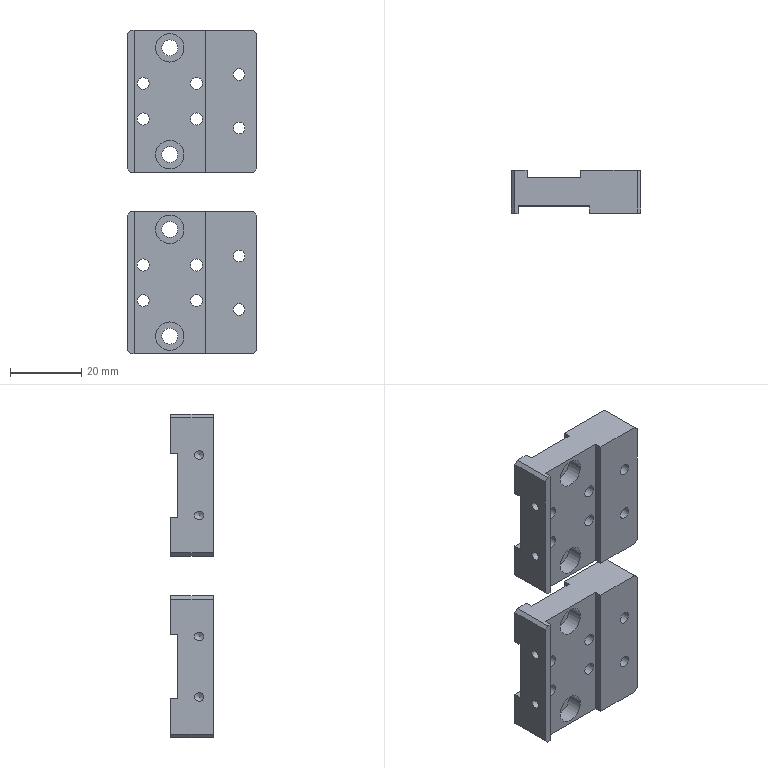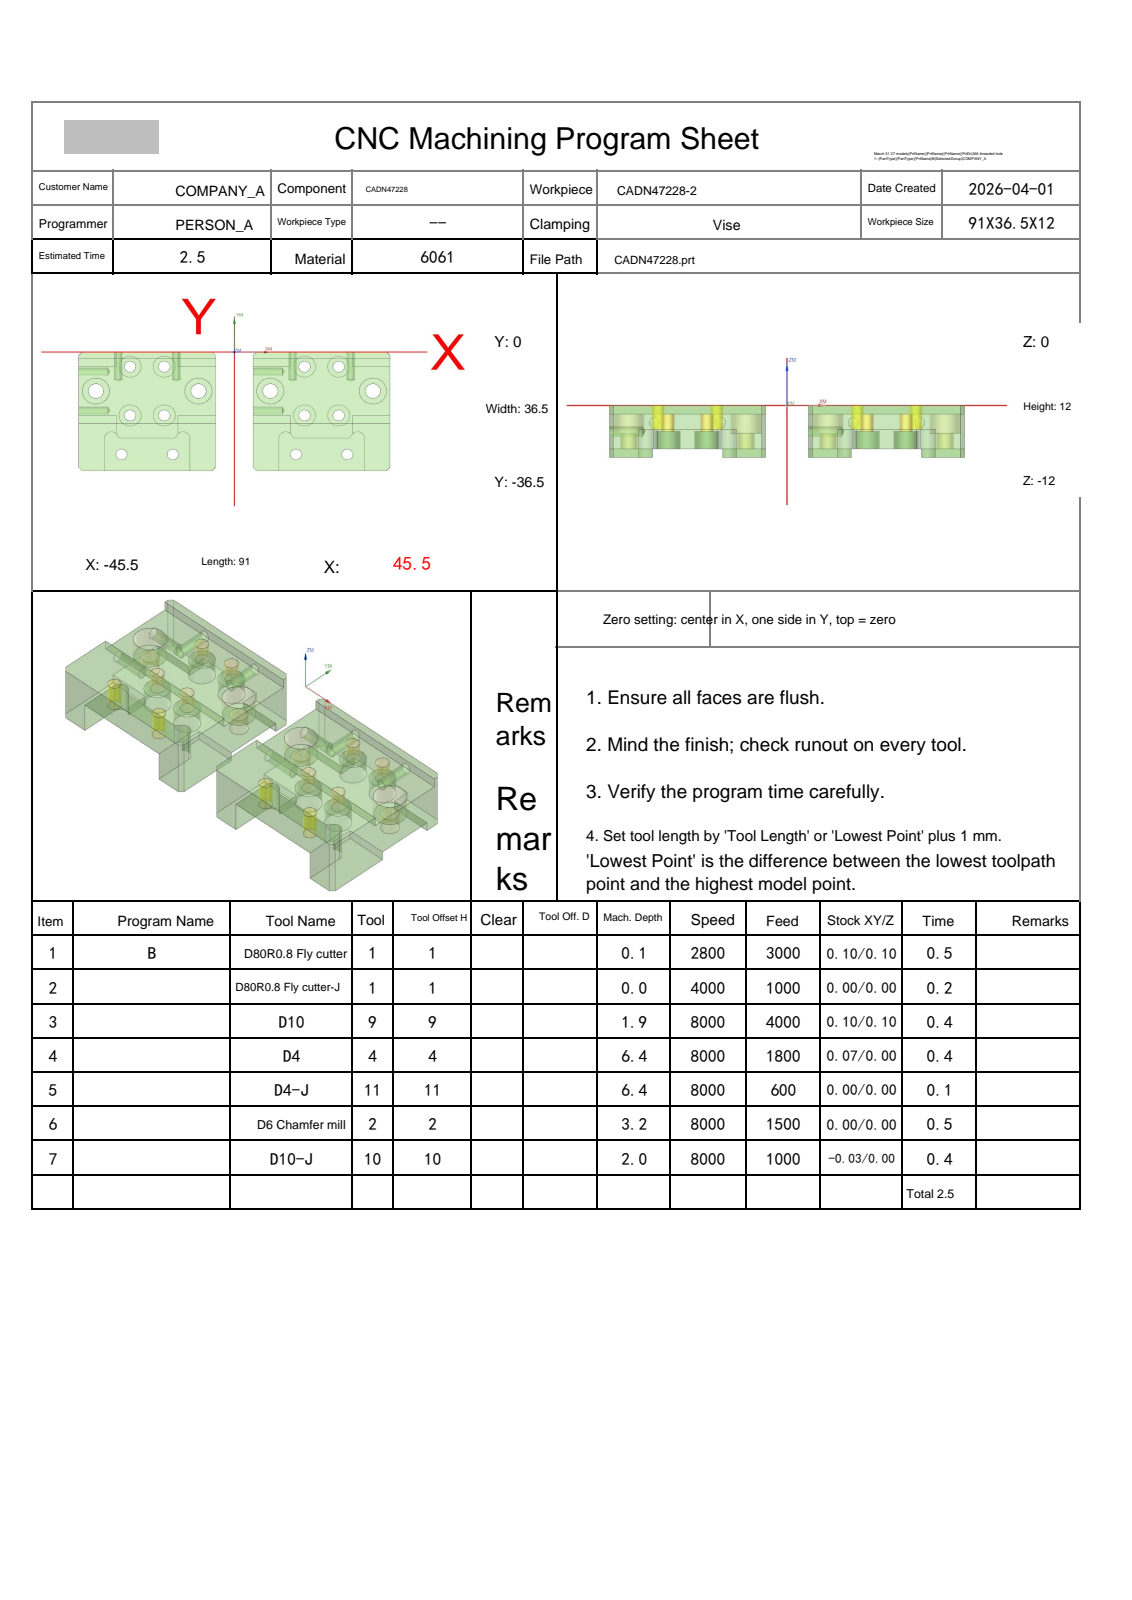NC program | NX | posted by the shop | part box 36.5 x 12 x 91 mm
Whole program:
%
O0001
(Machine time: 4.05 MIN)
(===Total Tool:6===)
(T1=D80R0.8 Fly cutter D=80.  R=0.8  D-  H01 Z=-0.   )
(T9=D10     D=10.  R=0.   D-  H09 Z=-1.9  )
(T4=D4      D=4.   R=0.   D-  H04 Z=-6.4  )
(T11=D4-J   D=4.   R=0.   D-  H11 Z=-6.4  )
(T2=D6 Chamfer mill   D=6.   R=0.   D-  H02 Z=-3.2  )
(T10=D10-J  D=10.  R=0.   D10 H10 Z=-2.   )
G80 G90 G17 G49 G40
G91 G28 Z0
M01
N1 T01 M06
(D80R0.8 Fly cutter  D=80. R=0.8 H=01 ce=0.10 di=0.10)
G00 G90 G54 X-97.597 Y-18.25 M03 S2800
G43 H01 Z20.
M08
Z4.517
G01 Z2.517 F3000.
X-85.597
X85.597
X97.597
Z4.517
G00 X-97.597
Z4.033
G01 Z2.033
X-85.597
X85.597
X97.597
Z4.033
G00 X-97.597
Z3.55
G01 Z1.55
X-85.597
X85.597
X97.597
Z3.55
G00 X-97.597
Z3.067
G01 Z1.067
X-85.597
X85.597
X97.597
Z3.067
G00 Z20.
X-97.597
Z2.583
G01 Z.583
X-85.597
X85.597
X97.597
Z2.583
G00 Z20.
X-97.597
Z2.1
G01 Z.1
X-85.597
X85.597
X97.597
Z2.1
G00 Z20.
G91 G28 Z0.0
M05
M09
G91 G28 Z0.0
M01
N2 T01 M06
(D80R0.8 Fly cutter-J  D=80. R=0.8 H=01 ce=0.00 di=0.00)
G00 G90 G54 X-97.499 Y-18.25 M03 S4000
G43 H01 Z20.
M08
Z2.
G01 Z0.0 F1000.
X-85.499
X85.499
X97.499
Z2.
G00 Z20.
G91 G28 Z0.0
M05
M09
G91 G28 Z0.0
M01
N3 T09 M06
(D10  D=10. R=0. H=09 ce=0.10 di=0.10)
G00 G90 G54 X-53.5 Y-12. M03 S8000
G43 H09 Z12.8
M08
Z1.025
G01 Z-.475 F4000.
X-50.4
Y-7.1
X50.4
Y-16.9
X-50.4
Y-14.868
G02 X-49.848 Y-13.974 I1. J0.0
G01 X-46.253 Y-12.175
G03 X-45.843 Y-11.795 I-.448 J.894
G02 X-45.502 Y-11.6 I.343 J-.205
G01 X45.502
G02 X45.9 Y-12. I-.002 J-.4
X45.502 Y-12.4 I-.4 J0.0
G01 X-45.502
G02 X-45.9 Y-12. I.002 J.4
G01 Y-11.998
G02 X-45.626 Y-11.62 I.4 J-.002
G01 X-46.572 Y-8.773
X-53.6
Z1.025
G00 X-53.5 Y-12.
Z.55
G01 Z-.95
X-50.4
Y-7.1
X50.4
Y-16.9
X-50.4
Y-14.868
G02 X-49.848 Y-13.974 I1. J0.0
G01 X-46.253 Y-12.175
G03 X-45.843 Y-11.795 I-.448 J.894
G02 X-45.502 Y-11.6 I.343 J-.205
G01 X45.502
G02 X45.9 Y-12. I-.002 J-.4
X45.502 Y-12.4 I-.4 J0.0
G01 X-45.502
G02 X-45.9 Y-12. I.002 J.4
G01 Y-11.998
G02 X-45.626 Y-11.62 I.4 J-.002
G01 X-46.572 Y-8.773
X-53.6
Z.55
G00 X-53.5 Y-12.
Z.075
G01 Z-1.425
X-50.4
Y-7.1
X50.4
Y-16.9
X-50.4
Y-14.868
G02 X-49.848 Y-13.974 I1. J0.0
G01 X-46.253 Y-12.175
G03 X-45.843 Y-11.795 I-.448 J.894
G02 X-45.502 Y-11.6 I.343 J-.205
G01 X45.502
G02 X45.9 Y-12. I-.002 J-.4
X45.502 Y-12.4 I-.4 J0.0
G01 X-45.502
G02 X-45.9 Y-12. I.002 J.4
G01 Y-11.998
G02 X-45.626 Y-11.62 I.4 J-.002
G01 X-46.572 Y-8.773
X-53.6
Z.075
G00 X-53.5 Y-12.
Z-.4
G01 Z-1.9
X-50.4
Y-7.1
X50.4
Y-16.9
X-50.4
Y-14.868
G02 X-49.848 Y-13.974 I1. J0.0
G01 X-46.253 Y-12.175
G03 X-45.843 Y-11.795 I-.448 J.894
G02 X-45.502 Y-11.6 I.343 J-.205
G01 X45.502
G02 X45.9 Y-12. I-.002 J-.4
X45.502 Y-12.4 I-.4 J0.0
G01 X-45.502
G02 X-45.9 Y-12. I.002 J.4
G01 Y-11.998
G02 X-45.626 Y-11.62 I.4 J-.002
G01 X-46.572 Y-8.773
X-53.6
Z-.4
G00 Z12.8
G91 G28 Z0.0
M05
M09
G91 G28 Z0.0
M01
N4 T04 M06
(D4  D=4. R=0. H=04 ce=0.07 di=0.00)
G00 G90 G54 X-10.5 Y-12. M03 S8000
G43 H04 Z20.
M08
Z-1.7
G03 X-11.465 Y-12.965 I0.0 J-.965 F1800.
X-10.5 Y-13.93 I.965 J0.0
X-10.5 Y-13.93 Z-2.05 I0.0 J1.93
X-10.5 Y-13.93 Z-2.4 I0.0 J1.93
X-10.5 Y-13.93 Z-2.75 I0.0 J1.93
X-10.5 Y-13.93 Z-3.1 I0.0 J1.93
X-10.5 Y-13.93 Z-3.45 I0.0 J1.93
X-10.5 Y-13.93 Z-3.8 I0.0 J1.93
X-10.5 Y-13.93 Z-4.15 I0.0 J1.93
X-10.5 Y-13.93 Z-4.5 I0.0 J1.93
X-10.5 Y-13.93 Z-4.85 I0.0 J1.93
X-10.5 Y-13.93 Z-5.2 I0.0 J1.93
X-10.5 Y-13.93 Z-5.55 I0.0 J1.93
X-10.5 Y-13.93 Z-5.9 I0.0 J1.93
X-10.5 Y-13.93 Z-6.25 I0.0 J1.93
X-9.663 Y-10.261 Z-6.4 I0.0 J1.93
X-10.5 Y-10.07 I-.837 J-1.739
X-12.43 Y-12. I0.0 J-1.93
X-10.5 Y-13.93 I1.93 J0.0
X-8.57 Y-12. I0.0 J1.93
X-9.663 Y-10.261 I-1.93 J0.0
X-10.081 Y-10.166 I-.419 J-.869
X-11.046 Y-11.131 I0.0 J-.965
X-10.5 Y-12. I.965 J0.0
G00 Z20.
X-40.5
Z-1.7
G03 X-41.465 Y-12.965 I0.0 J-.965
X-40.5 Y-13.93 I.965 J0.0
X-40.5 Y-13.93 Z-2.05 I0.0 J1.93
X-40.5 Y-13.93 Z-2.4 I0.0 J1.93
X-40.5 Y-13.93 Z-2.75 I0.0 J1.93
X-40.5 Y-13.93 Z-3.1 I0.0 J1.93
X-40.5 Y-13.93 Z-3.45 I0.0 J1.93
X-40.5 Y-13.93 Z-3.8 I0.0 J1.93
X-40.5 Y-13.93 Z-4.15 I0.0 J1.93
X-40.5 Y-13.93 Z-4.5 I0.0 J1.93
X-40.5 Y-13.93 Z-4.85 I0.0 J1.93
X-40.5 Y-13.93 Z-5.2 I0.0 J1.93
X-40.5 Y-13.93 Z-5.55 I0.0 J1.93
X-40.5 Y-13.93 Z-5.9 I0.0 J1.93
X-40.5 Y-13.93 Z-6.25 I0.0 J1.93
X-39.663 Y-10.261 Z-6.4 I0.0 J1.93
X-40.5 Y-10.07 I-.837 J-1.739
X-42.43 Y-12. I0.0 J-1.93
X-40.5 Y-13.93 I1.93 J0.0
X-38.57 Y-12. I0.0 J1.93
X-39.663 Y-10.261 I-1.93 J0.0
X-40.081 Y-10.166 I-.419 J-.869
X-41.046 Y-11.131 I0.0 J-.965
X-40.5 Y-12. I.965 J0.0
G00 Z20.
X10.5
Z-1.7
G03 X9.535 Y-12.965 I0.0 J-.965
X10.5 Y-13.93 I.965 J0.0
X10.5 Y-13.93 Z-2.05 I0.0 J1.93
X10.5 Y-13.93 Z-2.4 I0.0 J1.93
X10.5 Y-13.93 Z-2.75 I0.0 J1.93
X10.5 Y-13.93 Z-3.1 I0.0 J1.93
X10.5 Y-13.93 Z-3.45 I0.0 J1.93
X10.5 Y-13.93 Z-3.8 I0.0 J1.93
X10.5 Y-13.93 Z-4.15 I0.0 J1.93
X10.5 Y-13.93 Z-4.5 I0.0 J1.93
X10.5 Y-13.93 Z-4.85 I0.0 J1.93
X10.5 Y-13.93 Z-5.2 I0.0 J1.93
X10.5 Y-13.93 Z-5.55 I0.0 J1.93
X10.5 Y-13.93 Z-5.9 I0.0 J1.93
X10.5 Y-13.93 Z-6.25 I0.0 J1.93
X11.337 Y-10.261 Z-6.4 I0.0 J1.93
X10.5 Y-10.07 I-.837 J-1.739
X8.57 Y-12. I0.0 J-1.93
X10.5 Y-13.93 I1.93 J0.0
X12.43 Y-12. I0.0 J1.93
X11.337 Y-10.261 I-1.93 J0.0
X10.919 Y-10.166 I-.419 J-.869
X9.954 Y-11.131 I0.0 J-.965
X10.5 Y-12. I.965 J0.0
G00 Z20.
X40.5
Z-1.7
G03 X39.535 Y-12.965 I0.0 J-.965
X40.5 Y-13.93 I.965 J0.0
X40.5 Y-13.93 Z-2.05 I0.0 J1.93
X40.5 Y-13.93 Z-2.4 I0.0 J1.93
X40.5 Y-13.93 Z-2.75 I0.0 J1.93
X40.5 Y-13.93 Z-3.1 I0.0 J1.93
X40.5 Y-13.93 Z-3.45 I0.0 J1.93
X40.5 Y-13.93 Z-3.8 I0.0 J1.93
X40.5 Y-13.93 Z-4.15 I0.0 J1.93
X40.5 Y-13.93 Z-4.5 I0.0 J1.93
X40.5 Y-13.93 Z-4.85 I0.0 J1.93
X40.5 Y-13.93 Z-5.2 I0.0 J1.93
X40.5 Y-13.93 Z-5.55 I0.0 J1.93
X40.5 Y-13.93 Z-5.9 I0.0 J1.93
X40.5 Y-13.93 Z-6.25 I0.0 J1.93
X41.337 Y-10.261 Z-6.4 I0.0 J1.93
X40.5 Y-10.07 I-.837 J-1.739
X38.57 Y-12. I0.0 J-1.93
X40.5 Y-13.93 I1.93 J0.0
X42.43 Y-12. I0.0 J1.93
X41.337 Y-10.261 I-1.93 J0.0
X40.919 Y-10.166 I-.419 J-.869
X39.954 Y-11.131 I0.0 J-.965
X40.5 Y-12. I.965 J0.0
G00 Z20.
G91 G28 Z0.0
M05
M09
G91 G28 Z0.0
M01
N5 T11 M06
(D4-J  D=4. R=0. H=11 ce=0.00 di=0.00)
G00 G90 G54 X-10.5 Y-12. M03 S8000
G43 H11 Z20.
M08
Z-6.4
G01 X-10.829 Y-13.596 F600.
X-10.836 Y-13.664
G03 X-10.5 Y-14. I.336 J0.0
X-8.5 Y-12. I0.0 J2.
X-10.5 Y-10. I-2. J0.0
X-12.5 Y-12. I0.0 J-2.
X-10.5 Y-14. I2. J0.0
X-10.005 Y-13.938 I0.0 J2.
X-9.752 Y-13.612 I-.083 J.325
G01 X-9.786 Y-13.465
X-10.5 Y-12.
G00 Z20.
X-40.5
Z-6.4
G01 X-40.829 Y-13.596
X-40.836 Y-13.664
G03 X-40.5 Y-14. I.336 J0.0
X-38.5 Y-12. I0.0 J2.
X-40.5 Y-10. I-2. J0.0
X-42.5 Y-12. I0.0 J-2.
X-40.5 Y-14. I2. J0.0
X-40.005 Y-13.938 I0.0 J2.
X-39.752 Y-13.612 I-.083 J.325
G01 X-39.786 Y-13.465
X-40.5 Y-12.
G00 Z20.
X10.5
Z-6.4
G01 X10.171 Y-13.596
X10.164 Y-13.664
G03 X10.5 Y-14. I.336 J0.0
X12.5 Y-12. I0.0 J2.
X10.5 Y-10. I-2. J0.0
X8.5 Y-12. I0.0 J-2.
X10.5 Y-14. I2. J0.0
X10.995 Y-13.938 I0.0 J2.
X11.248 Y-13.612 I-.083 J.325
G01 X11.214 Y-13.465
X10.5 Y-12.
G00 Z20.
X40.5
Z-6.4
G01 X40.171 Y-13.596
X40.164 Y-13.664
G03 X40.5 Y-14. I.336 J0.0
X42.5 Y-12. I0.0 J2.
X40.5 Y-10. I-2. J0.0
X38.5 Y-12. I0.0 J-2.
X40.5 Y-14. I2. J0.0
X40.995 Y-13.938 I0.0 J2.
X41.248 Y-13.612 I-.083 J.325
G01 X41.214 Y-13.465
X40.5 Y-12.
G00 Z20.
G91 G28 Z0.0
M05
M09
G91 G28 Z0.0
M01
N6 T02 M06
(D6 Chamfer mill  D=6. R=0. H=02 ce=0.00 di=0.00)
G00 G90 G54 X-33. Y-31.5 M03 S8000
G43 H02 Z20.
M08
G98 G81 X-33. Y-31.5 Z-2.2 R3. F1000.
X-18.
X18.
X33.
G80
G00 Z20.
G00 G90 X-25.886 Y-20.773 M03 S6500
Z20.
Z.172
G01 Z-1.2 F1500.
G03 X-25.6 Y-20.973 I1.286 J1.532
G01 X-25.554 Y-21.003
X-25.5 Y-21.
X-5.5
G02 X-4.5 Y-22. I0.0 J-1.
G01 Y-35.5
X-4.534 Y-35.759
X-4.634 Y-36.
X-4.793 Y-36.207
X-5.793 Y-37.207
X-6. Y-37.366
X-6.241 Y-37.466
X-6.5 Y-37.5
X-44.5
X-44.759 Y-37.466
X-45. Y-37.366
X-45.207 Y-37.207
X-46.207 Y-36.207
X-46.366 Y-36.
X-46.466 Y-35.759
X-46.5 Y-35.5
Y-22.
G02 X-45.5 Y-21. I1. J0.0
G01 X-25.5
X-25.446 Y-21.003
X-25.4 Y-20.973
G03 X-25.114 Y-20.773 I-1. J1.732
G01 Z.172
G00 Z10.
X-32.506 Y-31.919
Z.405
G01 Z-1.2
G03 X-32.359 Y-31.603 I-1.732 J1.
G01 X-32.338 Y-31.553
X-32.35 Y-31.5
G03 X-33. Y-30.85 I-.65 J0.0
X-33.65 Y-31.5 I0.0 J-.65
X-33. Y-32.15 I.65 J0.0
X-32.35 Y-31.5 I0.0 J.65
G01 X-32.338 Y-31.447
X-32.359 Y-31.397
G03 X-32.506 Y-31.081 I-1.879 J-.684
G01 Z.405
G00 Z10.
X-17.506 Y-31.919
Z.405
G01 Z-1.2
G03 X-17.359 Y-31.603 I-1.732 J1.
G01 X-17.338 Y-31.553
X-17.35 Y-31.5
G03 X-18. Y-30.85 I-.65 J0.0
X-18.65 Y-31.5 I0.0 J-.65
X-18. Y-32.15 I.65 J0.0
X-17.35 Y-31.5 I0.0 J.65
G01 X-17.338 Y-31.447
X-17.359 Y-31.397
G03 X-17.506 Y-31.081 I-1.879 J-.684
G01 Z.405
G00 Z10.
X-25.114 Y-3.227
Z.172
G01 Z-1.2
G03 X-25.4 Y-3.027 I-1.286 J-1.532
G01 X-25.446 Y-2.997
X-25.5 Y-3.
X-45.5
G02 X-46.5 Y-2. I0.0 J1.
G01 Y-1.
X-46.466 Y-.741
X-46.366 Y-.5
X-46.207 Y-.293
X-45.207 Y.707
X-45. Y.866
X-44.759 Y.966
X-44.5 Y1.
X-6.5
X-6.241 Y.966
X-6. Y.866
X-5.793 Y.707
X-4.793 Y-.293
X-4.634 Y-.5
X-4.534 Y-.741
X-4.5 Y-1.
Y-2.
G02 X-5.5 Y-3. I-1. J0.0
G01 X-25.5
X-25.554 Y-2.997
X-25.6 Y-3.027
G03 X-25.886 Y-3.227 I1. J-1.732
G01 Z.172
G00 Z10.
X25.114 Y-20.773
Z.172
G01 Z-1.2
G03 X25.4 Y-20.973 I1.286 J1.532
G01 X25.446 Y-21.003
X25.5 Y-21.
X45.5
G02 X46.5 Y-22. I0.0 J-1.
G01 Y-35.5
X46.466 Y-35.759
X46.366 Y-36.
X46.207 Y-36.207
X45.207 Y-37.207
X45. Y-37.366
X44.759 Y-37.466
X44.5 Y-37.5
X6.5
X6.241 Y-37.466
X6. Y-37.366
X5.793 Y-37.207
X4.793 Y-36.207
X4.634 Y-36.
X4.534 Y-35.759
X4.5 Y-35.5
Y-22.
G02 X5.5 Y-21. I1. J0.0
G01 X25.5
X25.554 Y-21.003
X25.6 Y-20.973
G03 X25.886 Y-20.773 I-1. J1.732
G01 Z.172
G00 Z10.
X18.494 Y-31.919
Z.405
G01 Z-1.2
G03 X18.641 Y-31.603 I-1.732 J1.
G01 X18.662 Y-31.553
X18.65 Y-31.5
G03 X18. Y-30.85 I-.65 J0.0
X17.35 Y-31.5 I0.0 J-.65
X18. Y-32.15 I.65 J0.0
X18.65 Y-31.5 I0.0 J.65
G01 X18.662 Y-31.447
X18.641 Y-31.397
G03 X18.494 Y-31.081 I-1.879 J-.684
G01 Z.405
G00 Z10.
X33.494 Y-31.919
Z.405
G01 Z-1.2
G03 X33.641 Y-31.603 I-1.732 J1.
G01 X33.662 Y-31.553
X33.65 Y-31.5
G03 X33. Y-30.85 I-.65 J0.0
X32.35 Y-31.5 I0.0 J-.65
X33. Y-32.15 I.65 J0.0
X33.65 Y-31.5 I0.0 J.65
G01 X33.662 Y-31.447
X33.641 Y-31.397
G03 X33.494 Y-31.081 I-1.879 J-.684
G01 Z.405
G00 Z10.
X25.886 Y-3.227
Z.172
G01 Z-1.2
G03 X25.6 Y-3.027 I-1.286 J-1.532
G01 X25.554 Y-2.997
X25.5 Y-3.
X5.5
G02 X4.5 Y-2. I0.0 J1.
G01 Y-1.
X4.534 Y-.741
X4.634 Y-.5
X4.793 Y-.293
X5.793 Y.707
X6. Y.866
X6.241 Y.966
X6.5 Y1.
X44.5
X44.759 Y.966
X45. Y.866
X45.207 Y.707
X46.207 Y-.293
X46.366 Y-.5
X46.466 Y-.741
X46.5 Y-1.
Y-2.
G02 X45.5 Y-3. I-1. J0.0
G01 X25.5
X25.446 Y-2.997
X25.4 Y-3.027
G03 X25.114 Y-3.227 I1. J-1.732
G01 Z.172
G00 Z10.
X46.568 Y-4.97
Z-1.669
G01 Z-3.199
X46.508 Y-5.056
X46.5 Y-5.086
Y-18.914
X46.508 Y-18.944
X46.568 Y-19.03
Z-1.669
G00 Z10.
X4.432
Z-1.669
G01 Z-3.199
X4.492 Y-18.944
X4.5 Y-18.914
Y-5.086
X4.492 Y-5.056
X4.432 Y-4.97
Z-1.669
G00 Z.551
X7.697 Y-11.599
Z-1.767
G01 Z-3.199
G03 X7.519 Y-11.898 I1.624 J-1.167
G01 X7.493 Y-11.946
X7.5 Y-12.
G03 X10.5 Y-15. I3. J0.0
X13.5 Y-12. I0.0 J3.
X10.5 Y-9. I-3. J0.0
X7.5 Y-12. I0.0 J-3.
G01 X7.493 Y-12.054
X7.519 Y-12.102
G03 X7.697 Y-12.401 I1.802 J.868
G01 Z-1.767
G00 Z10.
X37.697 Y-11.599
Z-1.767
G01 Z-3.199
G03 X37.519 Y-11.898 I1.624 J-1.167
G01 X37.493 Y-11.946
X37.5 Y-12.
G03 X40.5 Y-15. I3. J0.0
X43.5 Y-12. I0.0 J3.
X40.5 Y-9. I-3. J0.0
X37.5 Y-12. I0.0 J-3.
G01 X37.493 Y-12.054
X37.519 Y-12.102
G03 X37.697 Y-12.401 I1.802 J.868
G01 Z-1.767
G00 Z10.
X-46.568 Y-19.03
Z-1.669
G01 Z-3.199
X-46.508 Y-18.944
X-46.5 Y-18.914
Y-5.086
X-46.508 Y-5.056
X-46.568 Y-4.97
Z-1.669
G00 Z10.
X-4.432
Z-1.669
G01 Z-3.199
X-4.492 Y-5.056
X-4.5 Y-5.086
Y-18.914
X-4.492 Y-18.944
X-4.432 Y-19.03
Z-1.669
G00 Z10.
X-43.303 Y-11.599
Z-1.767
G01 Z-3.199
G03 X-43.481 Y-11.898 I1.624 J-1.167
G01 X-43.507 Y-11.946
X-43.5 Y-12.
G03 X-40.5 Y-15. I3. J0.0
X-37.5 Y-12. I0.0 J3.
X-40.5 Y-9. I-3. J0.0
X-43.5 Y-12. I0.0 J-3.
G01 X-43.507 Y-12.054
X-43.481 Y-12.102
G03 X-43.303 Y-12.401 I1.802 J.868
G01 Z-1.767
G00 Z10.
X-13.303 Y-11.599
Z-1.767
G01 Z-3.199
G03 X-13.481 Y-11.898 I1.624 J-1.167
G01 X-13.507 Y-11.946
X-13.5 Y-12.
G03 X-10.5 Y-15. I3. J0.0
X-7.5 Y-12. I0.0 J3.
X-10.5 Y-9. I-3. J0.0
X-13.5 Y-12. I0.0 J-3.
G01 X-13.507 Y-12.054
X-13.481 Y-12.102
G03 X-13.303 Y-12.401 I1.802 J.868
G01 Z-1.767
G00 Z20.
G91 G28 Z0.0
M05
M09
G91 G28 Z0.0
M01
N7 T10 M06
(D10-J  D=10. R=0. H=10 ce=0.40 di=0.00)
G00 G90 G54 X-52.5 Y-14. M03 S8000
G43 H10 Z12.8
M08
Z-.5
G01 Z-2. F1000.
X-48.5
G03 X-46.5 Y-12. I0.0 J2.
G01 Y-8.397
G02 X-45.503 Y-7.4 I1. J-.003
G01 X45.503
G02 X46.5 Y-8.397 I-.003 J-1.
G01 Y-15.603
G02 X45.503 Y-16.6 I-1. J.003
G01 X-45.503
G02 X-46.5 Y-15.603 I.003 J1.
G01 Y-12.
Y-11.
G03 X-48.5 Y-9. I-2. J0.0
G01 X-52.9
Z-.5
G00 Z12.8
G00 G90 X-52.505 Y-15.178 M03 S8000
Z12.8
Z-1.
G01 Z-2. F1000.
G41 D10
X-52.47 Y-15.375
G03 X-50.5 Y-17.03 I1.97 J.345
G01 X50.5
G03 X52.47 Y-15.375 I0.0 J2.
G01 G40 X52.505 Y-15.178
Y-8.822
G41 D10
X52.47 Y-8.625
G03 X50.5 Y-6.97 I-1.97 J-.345
G01 X-50.5
G03 X-52.47 Y-8.625 I0.0 J-2.
G01 G40 X-52.505 Y-8.822
Z-1.
G00 Z12.8
M05
M09
G91 G28 Z0.0
G91 G28 Y0.0
M30
%